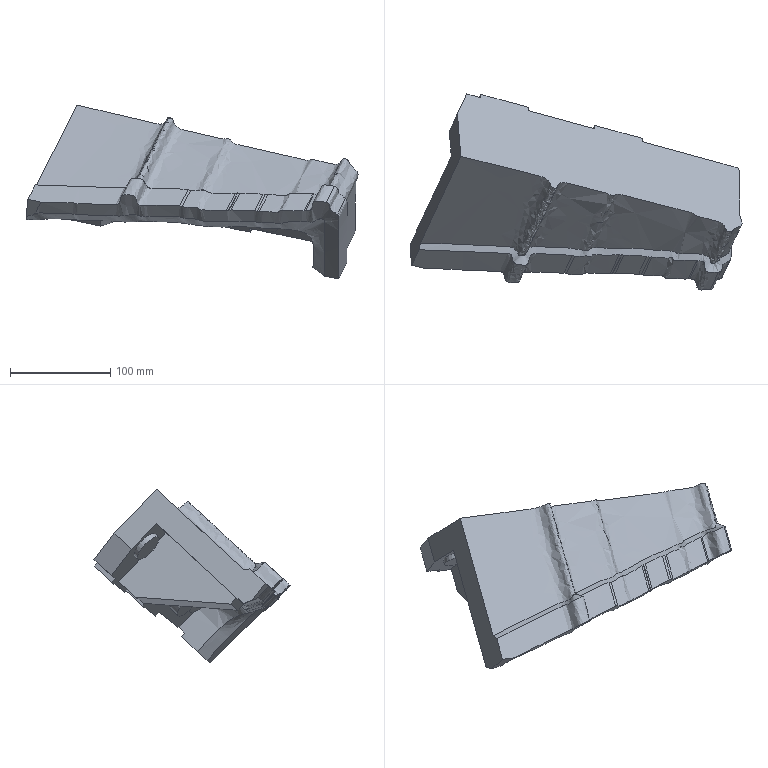Part | NX | features solid 2 | 1 solid | 50 faces | box 330.789 x 195.444 x 173.649 mm | volume 1695733 mm3 | plane 26 | spline 19 | cylinder 5 | commonest cylinder face diameters 30 x5